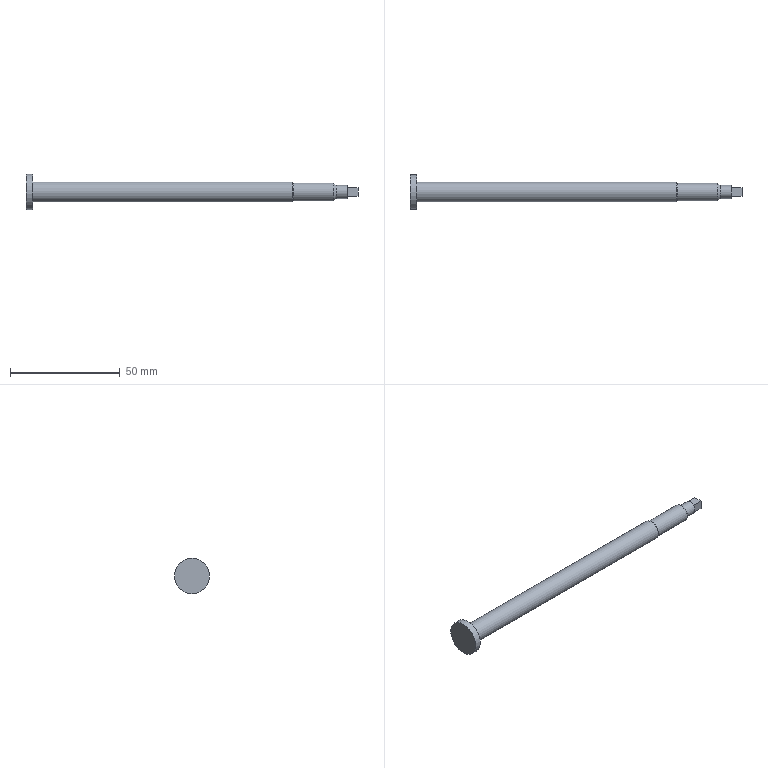Part | STEP file | Bolt | 1 solid | 14 faces | box 151 x 16 x 16 mm | volume 9327 mm3 | plane 8 | cylinder 4 | cone 1 | torus 1 | commonest cylinder face diameters 6 x1 8 x1 9 x1 16 x1
STEP:
#1=CARTESIAN_POINT('',(141.,0.,-3.));
#2=VERTEX_POINT('',#1);
#3=CARTESIAN_POINT('',(141.,0.,0.));
#4=DIRECTION('',(1.,0.,0.));
#5=DIRECTION('',(0.,0.,-1.));
#6=AXIS2_PLACEMENT_3D('',#3,#4,#5);
#7=CIRCLE('',#6,3.);
#8=EDGE_CURVE('',#2,#2,#7,.T.);
#9=ORIENTED_EDGE('',*,*,#8,.F.);
#10=EDGE_LOOP('',(#9));
#11=FACE_OUTER_BOUND('',#10,.T.);
#12=CARTESIAN_POINT('',(140.,0.,-4.));
#13=VERTEX_POINT('',#12);
#14=CARTESIAN_POINT('',(140.,0.,0.));
#15=DIRECTION('',(1.,0.,0.));
#16=DIRECTION('',(0.,0.,-1.));
#17=AXIS2_PLACEMENT_3D('',#14,#15,#16);
#18=CIRCLE('',#17,4.);
#19=EDGE_CURVE('',#13,#13,#18,.T.);
#20=ORIENTED_EDGE('',*,*,#19,.T.);
#21=EDGE_LOOP('',(#20));
#22=FACE_OUTER_BOUND('',#21,.T.);
#23=CARTESIAN_POINT('',(140.5,0.,0.));
#24=DIRECTION('',(-1.,0.,0.));
#25=DIRECTION('',(0.,0.,1.));
#26=AXIS2_PLACEMENT_3D('',#23,#24,#25);
#27=CONICAL_SURFACE('',#26,3.5,0.7854);
#28=ADVANCED_FACE('',(#11,#22),#27,.T.);
#29=CARTESIAN_POINT('',(146.,2.,2.));
#30=VERTEX_POINT('',#29);
#31=CARTESIAN_POINT('',(146.,2.,-2.));
#32=VERTEX_POINT('',#31);
#33=CARTESIAN_POINT('',(146.,2.,2.));
#34=DIRECTION('',(0.,0.,-1.));
#35=VECTOR('',#34,1.);
#36=LINE('',#33,#35);
#37=EDGE_CURVE('',#30,#32,#36,.T.);
#38=ORIENTED_EDGE('',*,*,#37,.F.);
#39=CARTESIAN_POINT('',(151.,2.,2.));
#40=VERTEX_POINT('',#39);
#41=CARTESIAN_POINT('',(146.,2.,2.));
#42=DIRECTION('',(1.,0.,0.));
#43=VECTOR('',#42,1.);
#44=LINE('',#41,#43);
#45=EDGE_CURVE('',#30,#40,#44,.T.);
#46=ORIENTED_EDGE('',*,*,#45,.T.);
#47=CARTESIAN_POINT('',(151.,2.,-2.));
#48=VERTEX_POINT('',#47);
#49=CARTESIAN_POINT('',(151.,2.,-2.));
#50=DIRECTION('',(0.,0.,1.));
#51=VECTOR('',#50,1.);
#52=LINE('',#49,#51);
#53=EDGE_CURVE('',#48,#40,#52,.T.);
#54=ORIENTED_EDGE('',*,*,#53,.F.);
#55=CARTESIAN_POINT('',(146.,2.,-2.));
#56=DIRECTION('',(1.,0.,0.));
#57=VECTOR('',#56,1.);
#58=LINE('',#55,#57);
#59=EDGE_CURVE('',#32,#48,#58,.T.);
#60=ORIENTED_EDGE('',*,*,#59,.F.);
#61=EDGE_LOOP('',(#38,#46,#54,#60));
#62=FACE_BOUND('',#61,.T.);
#63=CARTESIAN_POINT('',(141.,2.,-2.));
#64=DIRECTION('',(0.,1.,0.));
#65=DIRECTION('',(0.,0.,1.));
#66=AXIS2_PLACEMENT_3D('',#63,#64,#65);
#67=PLANE('',#66);
#68=ADVANCED_FACE('',(#62),#67,.T.);
#69=CARTESIAN_POINT('',(146.,-2.,2.));
#70=VERTEX_POINT('',#69);
#71=CARTESIAN_POINT('',(146.,-2.,2.));
#72=DIRECTION('',(0.,1.,0.));
#73=VECTOR('',#72,1.);
#74=LINE('',#71,#73);
#75=EDGE_CURVE('',#70,#30,#74,.T.);
#76=ORIENTED_EDGE('',*,*,#75,.F.);
#77=CARTESIAN_POINT('',(151.,-2.,2.));
#78=VERTEX_POINT('',#77);
#79=CARTESIAN_POINT('',(146.,-2.,2.));
#80=DIRECTION('',(1.,0.,0.));
#81=VECTOR('',#80,1.);
#82=LINE('',#79,#81);
#83=EDGE_CURVE('',#70,#78,#82,.T.);
#84=ORIENTED_EDGE('',*,*,#83,.T.);
#85=CARTESIAN_POINT('',(151.,2.,2.));
#86=DIRECTION('',(0.,-1.,0.));
#87=VECTOR('',#86,1.);
#88=LINE('',#85,#87);
#89=EDGE_CURVE('',#40,#78,#88,.T.);
#90=ORIENTED_EDGE('',*,*,#89,.F.);
#91=ORIENTED_EDGE('',*,*,#45,.F.);
#92=EDGE_LOOP('',(#76,#84,#90,#91));
#93=FACE_BOUND('',#92,.T.);
#94=CARTESIAN_POINT('',(141.,2.,2.));
#95=DIRECTION('',(0.,0.,1.));
#96=DIRECTION('',(0.,-1.,0.));
#97=AXIS2_PLACEMENT_3D('',#94,#95,#96);
#98=PLANE('',#97);
#99=ADVANCED_FACE('',(#93),#98,.T.);
#100=CARTESIAN_POINT('',(146.,-2.,-2.));
#101=VERTEX_POINT('',#100);
#102=CARTESIAN_POINT('',(146.,-2.,-2.));
#103=DIRECTION('',(0.,0.,1.));
#104=VECTOR('',#103,1.);
#105=LINE('',#102,#104);
#106=EDGE_CURVE('',#101,#70,#105,.T.);
#107=ORIENTED_EDGE('',*,*,#106,.F.);
#108=CARTESIAN_POINT('',(151.,-2.,-2.));
#109=VERTEX_POINT('',#108);
#110=CARTESIAN_POINT('',(146.,-2.,-2.));
#111=DIRECTION('',(1.,0.,0.));
#112=VECTOR('',#111,1.);
#113=LINE('',#110,#112);
#114=EDGE_CURVE('',#101,#109,#113,.T.);
#115=ORIENTED_EDGE('',*,*,#114,.T.);
#116=CARTESIAN_POINT('',(151.,-2.,2.));
#117=DIRECTION('',(0.,0.,-1.));
#118=VECTOR('',#117,1.);
#119=LINE('',#116,#118);
#120=EDGE_CURVE('',#78,#109,#119,.T.);
#121=ORIENTED_EDGE('',*,*,#120,.F.);
#122=ORIENTED_EDGE('',*,*,#83,.F.);
#123=EDGE_LOOP('',(#107,#115,#121,#122));
#124=FACE_BOUND('',#123,.T.);
#125=CARTESIAN_POINT('',(141.,-2.,2.));
#126=DIRECTION('',(0.,-1.,0.));
#127=DIRECTION('',(0.,0.,-1.));
#128=AXIS2_PLACEMENT_3D('',#125,#126,#127);
#129=PLANE('',#128);
#130=ADVANCED_FACE('',(#124),#129,.T.);
#131=CARTESIAN_POINT('',(146.,2.,-2.));
#132=DIRECTION('',(0.,-1.,0.));
#133=VECTOR('',#132,1.);
#134=LINE('',#131,#133);
#135=EDGE_CURVE('',#32,#101,#134,.T.);
#136=ORIENTED_EDGE('',*,*,#135,.F.);
#137=ORIENTED_EDGE('',*,*,#59,.T.);
#138=CARTESIAN_POINT('',(151.,-2.,-2.));
#139=DIRECTION('',(0.,1.,0.));
#140=VECTOR('',#139,1.);
#141=LINE('',#138,#140);
#142=EDGE_CURVE('',#109,#48,#141,.T.);
#143=ORIENTED_EDGE('',*,*,#142,.F.);
#144=ORIENTED_EDGE('',*,*,#114,.F.);
#145=EDGE_LOOP('',(#136,#137,#143,#144));
#146=FACE_BOUND('',#145,.T.);
#147=CARTESIAN_POINT('',(141.,-2.,-2.));
#148=DIRECTION('',(0.,0.,-1.));
#149=DIRECTION('',(0.,1.,0.));
#150=AXIS2_PLACEMENT_3D('',#147,#148,#149);
#151=PLANE('',#150);
#152=ADVANCED_FACE('',(#146),#151,.T.);
#153=CARTESIAN_POINT('',(146.,0.,-3.));
#154=VERTEX_POINT('',#153);
#155=CARTESIAN_POINT('',(146.,0.,0.));
#156=DIRECTION('',(1.,0.,0.));
#157=DIRECTION('',(0.,0.,-1.));
#158=AXIS2_PLACEMENT_3D('',#155,#156,#157);
#159=CIRCLE('',#158,3.);
#160=EDGE_CURVE('',#154,#154,#159,.T.);
#161=ORIENTED_EDGE('',*,*,#160,.F.);
#162=EDGE_LOOP('',(#161));
#163=FACE_OUTER_BOUND('',#162,.T.);
#164=ORIENTED_EDGE('',*,*,#8,.T.);
#165=EDGE_LOOP('',(#164));
#166=FACE_OUTER_BOUND('',#165,.T.);
#167=CARTESIAN_POINT('',(141.,0.,0.));
#168=DIRECTION('',(1.,0.,0.));
#169=DIRECTION('',(0.,0.,-1.));
#170=AXIS2_PLACEMENT_3D('',#167,#168,#169);
#171=CYLINDRICAL_SURFACE('',#170,3.);
#172=ADVANCED_FACE('',(#163,#166),#171,.T.);
#173=ORIENTED_EDGE('',*,*,#160,.T.);
#174=EDGE_LOOP('',(#173));
#175=FACE_BOUND('',#174,.T.);
#176=ORIENTED_EDGE('',*,*,#135,.T.);
#177=ORIENTED_EDGE('',*,*,#106,.T.);
#178=ORIENTED_EDGE('',*,*,#75,.T.);
#179=ORIENTED_EDGE('',*,*,#37,.T.);
#180=EDGE_LOOP('',(#176,#177,#178,#179));
#181=FACE_BOUND('',#180,.T.);
#182=CARTESIAN_POINT('',(146.,0.,-3.));
#183=DIRECTION('',(1.,0.,0.));
#184=DIRECTION('',(0.,1.,0.));
#185=AXIS2_PLACEMENT_3D('',#182,#183,#184);
#186=PLANE('',#185);
#187=ADVANCED_FACE('',(#175,#181),#186,.T.);
#188=ORIENTED_EDGE('',*,*,#19,.F.);
#189=EDGE_LOOP('',(#188));
#190=FACE_OUTER_BOUND('',#189,.T.);
#191=CARTESIAN_POINT('',(121.5,0.,-4.));
#192=VERTEX_POINT('',#191);
#193=CARTESIAN_POINT('',(121.5,0.,0.));
#194=DIRECTION('',(1.,0.,0.));
#195=DIRECTION('',(0.,0.,-1.));
#196=AXIS2_PLACEMENT_3D('',#193,#194,#195);
#197=CIRCLE('',#196,4.);
#198=EDGE_CURVE('',#192,#192,#197,.T.);
#199=ORIENTED_EDGE('',*,*,#198,.T.);
#200=EDGE_LOOP('',(#199));
#201=FACE_OUTER_BOUND('',#200,.T.);
#202=CARTESIAN_POINT('',(121.,0.,0.));
#203=DIRECTION('',(1.,0.,0.));
#204=DIRECTION('',(0.,0.,-1.));
#205=AXIS2_PLACEMENT_3D('',#202,#203,#204);
#206=CYLINDRICAL_SURFACE('',#205,4.);
#207=ADVANCED_FACE('',(#190,#201),#206,.T.);
#208=ORIENTED_EDGE('',*,*,#53,.T.);
#209=ORIENTED_EDGE('',*,*,#89,.T.);
#210=ORIENTED_EDGE('',*,*,#120,.T.);
#211=ORIENTED_EDGE('',*,*,#142,.T.);
#212=EDGE_LOOP('',(#208,#209,#210,#211));
#213=FACE_BOUND('',#212,.T.);
#214=CARTESIAN_POINT('',(151.,0.,0.));
#215=DIRECTION('',(1.,0.,0.));
#216=DIRECTION('',(0.,0.,-1.));
#217=AXIS2_PLACEMENT_3D('',#214,#215,#216);
#218=PLANE('',#217);
#219=ADVANCED_FACE('',(#213),#218,.T.);
#220=CARTESIAN_POINT('',(121.,0.,-4.5));
#221=VERTEX_POINT('',#220);
#222=CARTESIAN_POINT('',(121.,0.,0.));
#223=DIRECTION('',(1.,0.,0.));
#224=DIRECTION('',(0.,0.,-1.));
#225=AXIS2_PLACEMENT_3D('',#222,#223,#224);
#226=CIRCLE('',#225,4.5);
#227=EDGE_CURVE('',#221,#221,#226,.T.);
#228=ORIENTED_EDGE('',*,*,#227,.F.);
#229=EDGE_LOOP('',(#228));
#230=FACE_OUTER_BOUND('',#229,.T.);
#231=CARTESIAN_POINT('',(3.,0.,-4.5));
#232=VERTEX_POINT('',#231);
#233=CARTESIAN_POINT('',(3.,0.,0.));
#234=DIRECTION('',(1.,0.,0.));
#235=DIRECTION('',(0.,0.,-1.));
#236=AXIS2_PLACEMENT_3D('',#233,#234,#235);
#237=CIRCLE('',#236,4.5);
#238=EDGE_CURVE('',#232,#232,#237,.F.);
#239=ORIENTED_EDGE('',*,*,#238,.F.);
#240=EDGE_LOOP('',(#239));
#241=FACE_OUTER_BOUND('',#240,.T.);
#242=CARTESIAN_POINT('',(0.,0.,0.));
#243=DIRECTION('',(1.,0.,0.));
#244=DIRECTION('',(0.,0.,-1.));
#245=AXIS2_PLACEMENT_3D('',#242,#243,#244);
#246=CYLINDRICAL_SURFACE('',#245,4.5);
#247=ADVANCED_FACE('',(#230,#241),#246,.T.);
#248=CARTESIAN_POINT('',(3.,0.,-8.));
#249=VERTEX_POINT('',#248);
#250=CARTESIAN_POINT('',(3.,0.,0.));
#251=DIRECTION('',(1.,0.,0.));
#252=DIRECTION('',(0.,0.,-1.));
#253=AXIS2_PLACEMENT_3D('',#250,#251,#252);
#254=CIRCLE('',#253,8.);
#255=EDGE_CURVE('',#249,#249,#254,.T.);
#256=ORIENTED_EDGE('',*,*,#255,.T.);
#257=EDGE_LOOP('',(#256));
#258=FACE_BOUND('',#257,.T.);
#259=ORIENTED_EDGE('',*,*,#238,.T.);
#260=EDGE_LOOP('',(#259));
#261=FACE_BOUND('',#260,.T.);
#262=CARTESIAN_POINT('',(3.,0.,0.));
#263=DIRECTION('',(1.,0.,0.));
#264=DIRECTION('',(0.,0.,-1.));
#265=AXIS2_PLACEMENT_3D('',#262,#263,#264);
#266=PLANE('',#265);
#267=ADVANCED_FACE('',(#258,#261),#266,.T.);
#268=ORIENTED_EDGE('',*,*,#255,.F.);
#269=EDGE_LOOP('',(#268));
#270=FACE_OUTER_BOUND('',#269,.T.);
#271=CARTESIAN_POINT('',(0.,0.,-8.));
#272=VERTEX_POINT('',#271);
#273=CARTESIAN_POINT('',(0.,0.,0.));
#274=DIRECTION('',(1.,0.,0.));
#275=DIRECTION('',(0.,0.,-1.));
#276=AXIS2_PLACEMENT_3D('',#273,#274,#275);
#277=CIRCLE('',#276,8.);
#278=EDGE_CURVE('',#272,#272,#277,.T.);
#279=ORIENTED_EDGE('',*,*,#278,.T.);
#280=EDGE_LOOP('',(#279));
#281=FACE_OUTER_BOUND('',#280,.T.);
#282=CARTESIAN_POINT('',(0.,0.,0.));
#283=DIRECTION('',(1.,0.,0.));
#284=DIRECTION('',(0.,0.,-1.));
#285=AXIS2_PLACEMENT_3D('',#282,#283,#284);
#286=CYLINDRICAL_SURFACE('',#285,8.);
#287=ADVANCED_FACE('',(#270,#281),#286,.T.);
#288=ORIENTED_EDGE('',*,*,#278,.F.);
#289=EDGE_LOOP('',(#288));
#290=FACE_BOUND('',#289,.T.);
#291=CARTESIAN_POINT('',(0.,0.,0.));
#292=DIRECTION('',(1.,0.,0.));
#293=DIRECTION('',(0.,0.,-1.));
#294=AXIS2_PLACEMENT_3D('',#291,#292,#293);
#295=PLANE('',#294);
#296=ADVANCED_FACE('',(#290),#295,.F.);
#297=ORIENTED_EDGE('',*,*,#198,.F.);
#298=EDGE_LOOP('',(#297));
#299=FACE_OUTER_BOUND('',#298,.T.);
#300=ORIENTED_EDGE('',*,*,#227,.T.);
#301=EDGE_LOOP('',(#300));
#302=FACE_OUTER_BOUND('',#301,.T.);
#303=CARTESIAN_POINT('',(121.5,0.,0.));
#304=DIRECTION('',(1.,0.,0.));
#305=DIRECTION('',(0.,0.,-1.));
#306=AXIS2_PLACEMENT_3D('',#303,#304,#305);
#307=TOROIDAL_SURFACE('',#306,4.5,0.5);
#308=ADVANCED_FACE('',(#299,#302),#307,.F.);
#309=CLOSED_SHELL('',(#28,#68,#99,#130,#152,#172,#187,#207,#219,#247,#267,#287,#296,#308));
#310=MANIFOLD_SOLID_BREP('',#309);
#311=(LENGTH_UNIT()NAMED_UNIT(*)SI_UNIT(.MILLI.,.METRE.));
#312=UNCERTAINTY_MEASURE_WITH_UNIT(LENGTH_MEASURE(0.00001),#311,'','');
#313=(NAMED_UNIT(*)PLANE_ANGLE_UNIT()SI_UNIT($,.RADIAN.));
#314=(NAMED_UNIT(*)SI_UNIT($,.STERADIAN.)SOLID_ANGLE_UNIT());
#315=(GEOMETRIC_REPRESENTATION_CONTEXT(3)GLOBAL_UNCERTAINTY_ASSIGNED_CONTEXT((#312))GLOBAL_UNIT_ASSIGNED_CONTEXT((#311,#313,#314))REPRESENTATION_CONTEXT('',''));
#316=ADVANCED_BREP_SHAPE_REPRESENTATION('',(#310),#315);